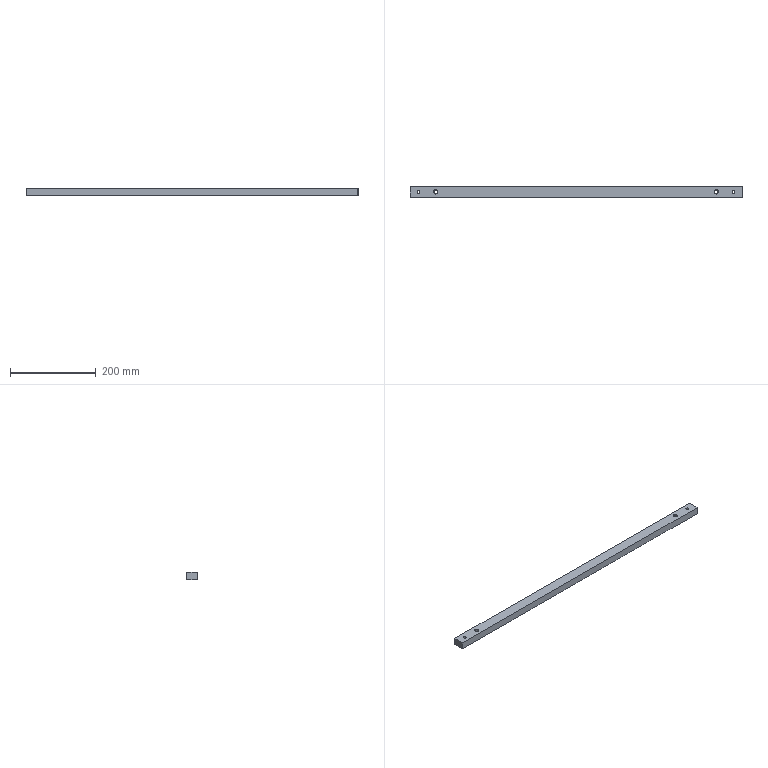Part | NX | features BREP 1 | 1 solid | 48 faces | box 774.5 x 26 x 17 mm | volume 338112 mm3 | cylinder 20 | cone 16 | plane 12 | commonest cylinder face diameters 3.3 x8 6.6 x4 8 x4 11 x4
STEP:
#1=CARTESIAN_POINT('',(372.75,0.,-1.5));
#2=VERTEX_POINT('',#1);
#3=CARTESIAN_POINT('',(361.75,0.,-1.5));
#4=VERTEX_POINT('',#3);
#5=CARTESIAN_POINT('',(367.25,0.,-1.5));
#6=DIRECTION('',(0.,0.,-1.));
#7=DIRECTION('',(-1.,0.,0.));
#8=AXIS2_PLACEMENT_3D('',#5,#6,#7);
#9=CIRCLE('',#8,5.5);
#10=EDGE_CURVE('',#2,#4,#9,.T.);
#11=ORIENTED_EDGE('',*,*,#10,.F.);
#12=CARTESIAN_POINT('',(372.75,0.,-8.5));
#13=VERTEX_POINT('',#12);
#14=CARTESIAN_POINT('',(372.75,0.,-8.5));
#15=DIRECTION('',(0.,0.,-1.));
#16=VECTOR('',#15,1000.);
#17=LINE('',#14,#16);
#18=EDGE_CURVE('',#2,#13,#17,.T.);
#19=ORIENTED_EDGE('',*,*,#18,.T.);
#20=CARTESIAN_POINT('',(361.75,0.,-8.5));
#21=VERTEX_POINT('',#20);
#22=CARTESIAN_POINT('',(367.25,0.,-8.5));
#23=DIRECTION('',(0.,0.,-1.));
#24=DIRECTION('',(-1.,0.,0.));
#25=AXIS2_PLACEMENT_3D('',#22,#23,#24);
#26=CIRCLE('',#25,5.5);
#27=EDGE_CURVE('',#13,#21,#26,.T.);
#28=ORIENTED_EDGE('',*,*,#27,.T.);
#29=CARTESIAN_POINT('',(361.75,0.,-8.5));
#30=DIRECTION('',(0.,0.,-1.));
#31=VECTOR('',#30,1000.);
#32=LINE('',#29,#31);
#33=EDGE_CURVE('',#4,#21,#32,.T.);
#34=ORIENTED_EDGE('',*,*,#33,.F.);
#35=EDGE_LOOP('',(#11,#19,#28,#34));
#36=FACE_BOUND('',#35,.T.);
#37=CARTESIAN_POINT('',(367.25,0.,-8.5));
#38=DIRECTION('',(0.,0.,-1.));
#39=DIRECTION('',(-1.,0.,0.));
#40=AXIS2_PLACEMENT_3D('',#37,#38,#39);
#41=CYLINDRICAL_SURFACE('',#40,5.5);
#42=ADVANCED_FACE('',(#36),#41,.F.);
#43=CARTESIAN_POINT('',(370.55,0.,8.5));
#44=VERTEX_POINT('',#43);
#45=CARTESIAN_POINT('',(363.95,0.,8.5));
#46=VERTEX_POINT('',#45);
#47=CARTESIAN_POINT('',(367.25,0.,8.5));
#48=DIRECTION('',(0.,0.,-1.));
#49=DIRECTION('',(-1.,0.,0.));
#50=AXIS2_PLACEMENT_3D('',#47,#48,#49);
#51=CIRCLE('',#50,3.3);
#52=EDGE_CURVE('',#44,#46,#51,.T.);
#53=ORIENTED_EDGE('',*,*,#52,.F.);
#54=CARTESIAN_POINT('',(370.55,0.,-1.5));
#55=VERTEX_POINT('',#54);
#56=CARTESIAN_POINT('',(370.55,0.,-8.5));
#57=DIRECTION('',(0.,0.,-1.));
#58=VECTOR('',#57,1000.);
#59=LINE('',#56,#58);
#60=EDGE_CURVE('',#44,#55,#59,.T.);
#61=ORIENTED_EDGE('',*,*,#60,.T.);
#62=CARTESIAN_POINT('',(363.95,0.,-1.5));
#63=VERTEX_POINT('',#62);
#64=CARTESIAN_POINT('',(367.25,0.,-1.5));
#65=DIRECTION('',(0.,0.,-1.));
#66=DIRECTION('',(-1.,0.,0.));
#67=AXIS2_PLACEMENT_3D('',#64,#65,#66);
#68=CIRCLE('',#67,3.3);
#69=EDGE_CURVE('',#55,#63,#68,.T.);
#70=ORIENTED_EDGE('',*,*,#69,.T.);
#71=CARTESIAN_POINT('',(363.95,0.,-8.5));
#72=DIRECTION('',(0.,0.,-1.));
#73=VECTOR('',#72,1000.);
#74=LINE('',#71,#73);
#75=EDGE_CURVE('',#46,#63,#74,.T.);
#76=ORIENTED_EDGE('',*,*,#75,.F.);
#77=EDGE_LOOP('',(#53,#61,#70,#76));
#78=FACE_BOUND('',#77,.T.);
#79=CARTESIAN_POINT('',(367.25,0.,-8.5));
#80=DIRECTION('',(0.,0.,-1.));
#81=DIRECTION('',(-1.,0.,0.));
#82=AXIS2_PLACEMENT_3D('',#79,#80,#81);
#83=CYLINDRICAL_SURFACE('',#82,3.3);
#84=ADVANCED_FACE('',(#78),#83,.F.);
#85=CARTESIAN_POINT('',(-361.75,0.,-1.5));
#86=VERTEX_POINT('',#85);
#87=CARTESIAN_POINT('',(-372.75,0.,-1.5));
#88=VERTEX_POINT('',#87);
#89=CARTESIAN_POINT('',(-367.25,0.,-1.5));
#90=DIRECTION('',(0.,0.,-1.));
#91=DIRECTION('',(-1.,0.,0.));
#92=AXIS2_PLACEMENT_3D('',#89,#90,#91);
#93=CIRCLE('',#92,5.5);
#94=EDGE_CURVE('',#86,#88,#93,.T.);
#95=ORIENTED_EDGE('',*,*,#94,.F.);
#96=CARTESIAN_POINT('',(-361.75,0.,-8.5));
#97=VERTEX_POINT('',#96);
#98=CARTESIAN_POINT('',(-361.75,0.,-8.5));
#99=DIRECTION('',(0.,0.,-1.));
#100=VECTOR('',#99,1000.);
#101=LINE('',#98,#100);
#102=EDGE_CURVE('',#86,#97,#101,.T.);
#103=ORIENTED_EDGE('',*,*,#102,.T.);
#104=CARTESIAN_POINT('',(-372.75,0.,-8.5));
#105=VERTEX_POINT('',#104);
#106=CARTESIAN_POINT('',(-367.25,0.,-8.5));
#107=DIRECTION('',(0.,0.,-1.));
#108=DIRECTION('',(-1.,0.,0.));
#109=AXIS2_PLACEMENT_3D('',#106,#107,#108);
#110=CIRCLE('',#109,5.5);
#111=EDGE_CURVE('',#97,#105,#110,.T.);
#112=ORIENTED_EDGE('',*,*,#111,.T.);
#113=CARTESIAN_POINT('',(-372.75,0.,-8.5));
#114=DIRECTION('',(0.,0.,-1.));
#115=VECTOR('',#114,1000.);
#116=LINE('',#113,#115);
#117=EDGE_CURVE('',#88,#105,#116,.T.);
#118=ORIENTED_EDGE('',*,*,#117,.F.);
#119=EDGE_LOOP('',(#95,#103,#112,#118));
#120=FACE_BOUND('',#119,.T.);
#121=CARTESIAN_POINT('',(-367.25,0.,-8.5));
#122=DIRECTION('',(0.,0.,-1.));
#123=DIRECTION('',(-1.,0.,0.));
#124=AXIS2_PLACEMENT_3D('',#121,#122,#123);
#125=CYLINDRICAL_SURFACE('',#124,5.5);
#126=ADVANCED_FACE('',(#120),#125,.F.);
#127=CARTESIAN_POINT('',(-363.95,0.,8.5));
#128=VERTEX_POINT('',#127);
#129=CARTESIAN_POINT('',(-370.55,0.,8.5));
#130=VERTEX_POINT('',#129);
#131=CARTESIAN_POINT('',(-367.25,0.,8.5));
#132=DIRECTION('',(0.,0.,-1.));
#133=DIRECTION('',(-1.,0.,0.));
#134=AXIS2_PLACEMENT_3D('',#131,#132,#133);
#135=CIRCLE('',#134,3.3);
#136=EDGE_CURVE('',#128,#130,#135,.T.);
#137=ORIENTED_EDGE('',*,*,#136,.F.);
#138=CARTESIAN_POINT('',(-363.95,0.,-1.5));
#139=VERTEX_POINT('',#138);
#140=CARTESIAN_POINT('',(-363.95,0.,-8.5));
#141=DIRECTION('',(0.,0.,-1.));
#142=VECTOR('',#141,1000.);
#143=LINE('',#140,#142);
#144=EDGE_CURVE('',#128,#139,#143,.T.);
#145=ORIENTED_EDGE('',*,*,#144,.T.);
#146=CARTESIAN_POINT('',(-370.55,0.,-1.5));
#147=VERTEX_POINT('',#146);
#148=CARTESIAN_POINT('',(-367.25,0.,-1.5));
#149=DIRECTION('',(0.,0.,-1.));
#150=DIRECTION('',(-1.,0.,0.));
#151=AXIS2_PLACEMENT_3D('',#148,#149,#150);
#152=CIRCLE('',#151,3.3);
#153=EDGE_CURVE('',#139,#147,#152,.T.);
#154=ORIENTED_EDGE('',*,*,#153,.T.);
#155=CARTESIAN_POINT('',(-370.55,0.,-8.5));
#156=DIRECTION('',(0.,0.,-1.));
#157=VECTOR('',#156,1000.);
#158=LINE('',#155,#157);
#159=EDGE_CURVE('',#130,#147,#158,.T.);
#160=ORIENTED_EDGE('',*,*,#159,.F.);
#161=EDGE_LOOP('',(#137,#145,#154,#160));
#162=FACE_BOUND('',#161,.T.);
#163=CARTESIAN_POINT('',(-367.25,0.,-8.5));
#164=DIRECTION('',(0.,0.,-1.));
#165=DIRECTION('',(-1.,0.,0.));
#166=AXIS2_PLACEMENT_3D('',#163,#164,#165);
#167=CYLINDRICAL_SURFACE('',#166,3.3);
#168=ADVANCED_FACE('',(#162),#167,.F.);
#169=CARTESIAN_POINT('',(-331.25,0.,7.5));
#170=VERTEX_POINT('',#169);
#171=CARTESIAN_POINT('',(-323.25,0.,7.5));
#172=VERTEX_POINT('',#171);
#173=CARTESIAN_POINT('',(-327.25,0.,7.5));
#174=DIRECTION('',(0.,0.,1.));
#175=DIRECTION('',(-1.,0.,0.));
#176=AXIS2_PLACEMENT_3D('',#173,#174,#175);
#177=CIRCLE('',#176,4.);
#178=EDGE_CURVE('',#170,#172,#177,.T.);
#179=ORIENTED_EDGE('',*,*,#178,.F.);
#180=CARTESIAN_POINT('',(-332.25,0.,8.5));
#181=VERTEX_POINT('',#180);
#182=CARTESIAN_POINT('',(-331.25,0.,7.5));
#183=DIRECTION('',(-0.7071,0.,0.7071));
#184=VECTOR('',#183,1000.);
#185=LINE('',#182,#184);
#186=EDGE_CURVE('',#181,#170,#185,.F.);
#187=ORIENTED_EDGE('',*,*,#186,.F.);
#188=CARTESIAN_POINT('',(-322.25,0.,8.5));
#189=VERTEX_POINT('',#188);
#190=CARTESIAN_POINT('',(-327.25,0.,8.5));
#191=DIRECTION('',(0.,0.,-1.));
#192=DIRECTION('',(-1.,0.,0.));
#193=AXIS2_PLACEMENT_3D('',#190,#191,#192);
#194=CIRCLE('',#193,5.);
#195=EDGE_CURVE('',#189,#181,#194,.T.);
#196=ORIENTED_EDGE('',*,*,#195,.F.);
#197=CARTESIAN_POINT('',(-323.25,0.,7.5));
#198=DIRECTION('',(0.7071,0.,0.7071));
#199=VECTOR('',#198,1000.);
#200=LINE('',#197,#199);
#201=EDGE_CURVE('',#189,#172,#200,.F.);
#202=ORIENTED_EDGE('',*,*,#201,.T.);
#203=EDGE_LOOP('',(#179,#187,#196,#202));
#204=FACE_BOUND('',#203,.T.);
#205=CARTESIAN_POINT('',(-327.25,0.,7.5));
#206=DIRECTION('',(0.,0.,1.));
#207=DIRECTION('',(1.,0.,0.));
#208=AXIS2_PLACEMENT_3D('',#205,#206,#207);
#209=CONICAL_SURFACE('',#208,4.,0.7854);
#210=ADVANCED_FACE('',(#204),#209,.F.);
#211=CARTESIAN_POINT('',(-323.25,0.,-7.5));
#212=VERTEX_POINT('',#211);
#213=CARTESIAN_POINT('',(-331.25,0.,-7.5));
#214=VERTEX_POINT('',#213);
#215=CARTESIAN_POINT('',(-327.25,0.,-7.5));
#216=DIRECTION('',(0.,0.,-1.));
#217=DIRECTION('',(-1.,0.,0.));
#218=AXIS2_PLACEMENT_3D('',#215,#216,#217);
#219=CIRCLE('',#218,4.);
#220=EDGE_CURVE('',#212,#214,#219,.T.);
#221=ORIENTED_EDGE('',*,*,#220,.F.);
#222=CARTESIAN_POINT('',(-322.25,0.,-8.5));
#223=VERTEX_POINT('',#222);
#224=CARTESIAN_POINT('',(-323.25,0.,-7.5));
#225=DIRECTION('',(0.7071,0.,-0.7071));
#226=VECTOR('',#225,1000.);
#227=LINE('',#224,#226);
#228=EDGE_CURVE('',#212,#223,#227,.T.);
#229=ORIENTED_EDGE('',*,*,#228,.T.);
#230=CARTESIAN_POINT('',(-332.25,0.,-8.5));
#231=VERTEX_POINT('',#230);
#232=CARTESIAN_POINT('',(-327.25,0.,-8.5));
#233=DIRECTION('',(0.,0.,1.));
#234=DIRECTION('',(-1.,0.,0.));
#235=AXIS2_PLACEMENT_3D('',#232,#233,#234);
#236=CIRCLE('',#235,5.);
#237=EDGE_CURVE('',#231,#223,#236,.T.);
#238=ORIENTED_EDGE('',*,*,#237,.F.);
#239=CARTESIAN_POINT('',(-331.25,0.,-7.5));
#240=DIRECTION('',(-0.7071,0.,-0.7071));
#241=VECTOR('',#240,1000.);
#242=LINE('',#239,#241);
#243=EDGE_CURVE('',#214,#231,#242,.T.);
#244=ORIENTED_EDGE('',*,*,#243,.F.);
#245=EDGE_LOOP('',(#221,#229,#238,#244));
#246=FACE_BOUND('',#245,.T.);
#247=CARTESIAN_POINT('',(-327.25,0.,-7.5));
#248=DIRECTION('',(0.,0.,-1.));
#249=DIRECTION('',(-1.,0.,0.));
#250=AXIS2_PLACEMENT_3D('',#247,#248,#249);
#251=CONICAL_SURFACE('',#250,4.,0.7854);
#252=ADVANCED_FACE('',(#246),#251,.F.);
#253=CARTESIAN_POINT('',(323.25,0.,7.5));
#254=VERTEX_POINT('',#253);
#255=CARTESIAN_POINT('',(331.25,0.,7.5));
#256=VERTEX_POINT('',#255);
#257=CARTESIAN_POINT('',(327.25,0.,7.5));
#258=DIRECTION('',(0.,0.,1.));
#259=DIRECTION('',(-1.,0.,0.));
#260=AXIS2_PLACEMENT_3D('',#257,#258,#259);
#261=CIRCLE('',#260,4.);
#262=EDGE_CURVE('',#254,#256,#261,.T.);
#263=ORIENTED_EDGE('',*,*,#262,.F.);
#264=CARTESIAN_POINT('',(322.25,0.,8.5));
#265=VERTEX_POINT('',#264);
#266=CARTESIAN_POINT('',(323.25,0.,7.5));
#267=DIRECTION('',(-0.7071,0.,0.7071));
#268=VECTOR('',#267,1000.);
#269=LINE('',#266,#268);
#270=EDGE_CURVE('',#265,#254,#269,.F.);
#271=ORIENTED_EDGE('',*,*,#270,.F.);
#272=CARTESIAN_POINT('',(332.25,0.,8.5));
#273=VERTEX_POINT('',#272);
#274=CARTESIAN_POINT('',(327.25,0.,8.5));
#275=DIRECTION('',(0.,0.,-1.));
#276=DIRECTION('',(-1.,0.,0.));
#277=AXIS2_PLACEMENT_3D('',#274,#275,#276);
#278=CIRCLE('',#277,5.);
#279=EDGE_CURVE('',#273,#265,#278,.T.);
#280=ORIENTED_EDGE('',*,*,#279,.F.);
#281=CARTESIAN_POINT('',(331.25,0.,7.5));
#282=DIRECTION('',(0.7071,0.,0.7071));
#283=VECTOR('',#282,1000.);
#284=LINE('',#281,#283);
#285=EDGE_CURVE('',#273,#256,#284,.F.);
#286=ORIENTED_EDGE('',*,*,#285,.T.);
#287=EDGE_LOOP('',(#263,#271,#280,#286));
#288=FACE_BOUND('',#287,.T.);
#289=CARTESIAN_POINT('',(327.25,0.,7.5));
#290=DIRECTION('',(0.,0.,1.));
#291=DIRECTION('',(1.,0.,0.));
#292=AXIS2_PLACEMENT_3D('',#289,#290,#291);
#293=CONICAL_SURFACE('',#292,4.,0.7854);
#294=ADVANCED_FACE('',(#288),#293,.F.);
#295=CARTESIAN_POINT('',(331.25,0.,-7.5));
#296=VERTEX_POINT('',#295);
#297=CARTESIAN_POINT('',(323.25,0.,-7.5));
#298=VERTEX_POINT('',#297);
#299=CARTESIAN_POINT('',(327.25,0.,-7.5));
#300=DIRECTION('',(0.,0.,-1.));
#301=DIRECTION('',(-1.,0.,0.));
#302=AXIS2_PLACEMENT_3D('',#299,#300,#301);
#303=CIRCLE('',#302,4.);
#304=EDGE_CURVE('',#296,#298,#303,.T.);
#305=ORIENTED_EDGE('',*,*,#304,.F.);
#306=CARTESIAN_POINT('',(332.25,0.,-8.5));
#307=VERTEX_POINT('',#306);
#308=CARTESIAN_POINT('',(331.25,0.,-7.5));
#309=DIRECTION('',(0.7071,0.,-0.7071));
#310=VECTOR('',#309,1000.);
#311=LINE('',#308,#310);
#312=EDGE_CURVE('',#296,#307,#311,.T.);
#313=ORIENTED_EDGE('',*,*,#312,.T.);
#314=CARTESIAN_POINT('',(322.25,0.,-8.5));
#315=VERTEX_POINT('',#314);
#316=CARTESIAN_POINT('',(327.25,0.,-8.5));
#317=DIRECTION('',(0.,0.,1.));
#318=DIRECTION('',(-1.,0.,0.));
#319=AXIS2_PLACEMENT_3D('',#316,#317,#318);
#320=CIRCLE('',#319,5.);
#321=EDGE_CURVE('',#315,#307,#320,.T.);
#322=ORIENTED_EDGE('',*,*,#321,.F.);
#323=CARTESIAN_POINT('',(323.25,0.,-7.5));
#324=DIRECTION('',(-0.7071,0.,-0.7071));
#325=VECTOR('',#324,1000.);
#326=LINE('',#323,#325);
#327=EDGE_CURVE('',#298,#315,#326,.T.);
#328=ORIENTED_EDGE('',*,*,#327,.F.);
#329=EDGE_LOOP('',(#305,#313,#322,#328));
#330=FACE_BOUND('',#329,.T.);
#331=CARTESIAN_POINT('',(327.25,0.,-7.5));
#332=DIRECTION('',(0.,0.,-1.));
#333=DIRECTION('',(-1.,0.,0.));
#334=AXIS2_PLACEMENT_3D('',#331,#332,#333);
#335=CONICAL_SURFACE('',#334,4.,0.7854);
#336=ADVANCED_FACE('',(#330),#335,.F.);
#337=ORIENTED_EDGE('',*,*,#304,.T.);
#338=CARTESIAN_POINT('',(323.25,0.,-174.5));
#339=DIRECTION('',(0.,0.,1.));
#340=VECTOR('',#339,1000.);
#341=LINE('',#338,#340);
#342=EDGE_CURVE('',#254,#298,#341,.F.);
#343=ORIENTED_EDGE('',*,*,#342,.F.);
#344=ORIENTED_EDGE('',*,*,#262,.T.);
#345=CARTESIAN_POINT('',(331.25,0.,-174.5));
#346=DIRECTION('',(0.,0.,1.));
#347=VECTOR('',#346,1000.);
#348=LINE('',#345,#347);
#349=EDGE_CURVE('',#256,#296,#348,.F.);
#350=ORIENTED_EDGE('',*,*,#349,.T.);
#351=EDGE_LOOP('',(#337,#343,#344,#350));
#352=FACE_BOUND('',#351,.T.);
#353=CARTESIAN_POINT('',(327.25,0.,-174.5));
#354=DIRECTION('',(0.,0.,1.));
#355=DIRECTION('',(1.,0.,0.));
#356=AXIS2_PLACEMENT_3D('',#353,#354,#355);
#357=CYLINDRICAL_SURFACE('',#356,4.);
#358=ADVANCED_FACE('',(#352),#357,.F.);
#359=ORIENTED_EDGE('',*,*,#220,.T.);
#360=CARTESIAN_POINT('',(-331.25,0.,-174.5));
#361=DIRECTION('',(0.,0.,1.));
#362=VECTOR('',#361,1000.);
#363=LINE('',#360,#362);
#364=EDGE_CURVE('',#170,#214,#363,.F.);
#365=ORIENTED_EDGE('',*,*,#364,.F.);
#366=ORIENTED_EDGE('',*,*,#178,.T.);
#367=CARTESIAN_POINT('',(-323.25,0.,-174.5));
#368=DIRECTION('',(0.,0.,1.));
#369=VECTOR('',#368,1000.);
#370=LINE('',#367,#369);
#371=EDGE_CURVE('',#172,#212,#370,.F.);
#372=ORIENTED_EDGE('',*,*,#371,.T.);
#373=EDGE_LOOP('',(#359,#365,#366,#372));
#374=FACE_BOUND('',#373,.T.);
#375=CARTESIAN_POINT('',(-327.25,0.,-174.5));
#376=DIRECTION('',(0.,0.,1.));
#377=DIRECTION('',(1.,0.,0.));
#378=AXIS2_PLACEMENT_3D('',#375,#376,#377);
#379=CYLINDRICAL_SURFACE('',#378,4.);
#380=ADVANCED_FACE('',(#374),#379,.F.);
#381=CARTESIAN_POINT('',(-374.25,1.5,-1.65));
#382=VERTEX_POINT('',#381);
#383=CARTESIAN_POINT('',(-374.25,1.5,1.65));
#384=VERTEX_POINT('',#383);
#385=CARTESIAN_POINT('',(-374.25,1.5,0.));
#386=DIRECTION('',(0.,1.,0.));
#387=DIRECTION('',(0.,0.,1.));
#388=AXIS2_PLACEMENT_3D('',#385,#386,#387);
#389=CIRCLE('',#388,1.65);
#390=EDGE_CURVE('',#382,#384,#389,.T.);
#391=ORIENTED_EDGE('',*,*,#390,.F.);
#392=CARTESIAN_POINT('',(-374.25,13.,-1.65));
#393=VERTEX_POINT('',#392);
#394=CARTESIAN_POINT('',(-374.25,13.,-1.65));
#395=DIRECTION('',(0.,1.,0.));
#396=VECTOR('',#395,1000.);
#397=LINE('',#394,#396);
#398=EDGE_CURVE('',#393,#382,#397,.F.);
#399=ORIENTED_EDGE('',*,*,#398,.F.);
#400=CARTESIAN_POINT('',(-374.25,13.,1.65));
#401=VERTEX_POINT('',#400);
#402=CARTESIAN_POINT('',(-374.25,13.,0.));
#403=DIRECTION('',(0.,1.,0.));
#404=DIRECTION('',(0.,0.,1.));
#405=AXIS2_PLACEMENT_3D('',#402,#403,#404);
#406=CIRCLE('',#405,1.65);
#407=EDGE_CURVE('',#393,#401,#406,.T.);
#408=ORIENTED_EDGE('',*,*,#407,.T.);
#409=CARTESIAN_POINT('',(-374.25,13.,1.65));
#410=DIRECTION('',(0.,1.,0.));
#411=VECTOR('',#410,1000.);
#412=LINE('',#409,#411);
#413=EDGE_CURVE('',#401,#384,#412,.F.);
#414=ORIENTED_EDGE('',*,*,#413,.T.);
#415=EDGE_LOOP('',(#391,#399,#408,#414));
#416=FACE_BOUND('',#415,.T.);
#417=CARTESIAN_POINT('',(-374.25,13.,0.));
#418=DIRECTION('',(0.,1.,0.));
#419=DIRECTION('',(0.,0.,1.));
#420=AXIS2_PLACEMENT_3D('',#417,#418,#419);
#421=CYLINDRICAL_SURFACE('',#420,1.65);
#422=ADVANCED_FACE('',(#416),#421,.F.);
#423=CARTESIAN_POINT('',(-374.25,0.5086,0.));
#424=VERTEX_POINT('',#423);
#425=CARTESIAN_POINT('',(-374.25,1.5,1.65));
#426=DIRECTION('',(0.,0.515,0.8572));
#427=VECTOR('',#426,1000.);
#428=LINE('',#425,#427);
#429=EDGE_CURVE('',#384,#424,#428,.F.);
#430=ORIENTED_EDGE('',*,*,#429,.T.);
#431=CARTESIAN_POINT('',(-374.25,1.5,-1.65));
#432=DIRECTION('',(0.,0.515,-0.8572));
#433=VECTOR('',#432,1000.);
#434=LINE('',#431,#433);
#435=EDGE_CURVE('',#382,#424,#434,.F.);
#436=ORIENTED_EDGE('',*,*,#435,.F.);
#437=ORIENTED_EDGE('',*,*,#390,.T.);
#438=EDGE_LOOP('',(#430,#436,#437));
#439=FACE_BOUND('',#438,.T.);
#440=CARTESIAN_POINT('',(-374.25,1.5,0.));
#441=DIRECTION('',(0.,1.,0.));
#442=DIRECTION('',(0.,0.,1.));
#443=AXIS2_PLACEMENT_3D('',#440,#441,#442);
#444=CONICAL_SURFACE('',#443,1.65,1.03);
#445=ADVANCED_FACE('',(#439),#444,.F.);
#446=CARTESIAN_POINT('',(-137.25,1.5,-1.65));
#447=VERTEX_POINT('',#446);
#448=CARTESIAN_POINT('',(-137.25,1.5,1.65));
#449=VERTEX_POINT('',#448);
#450=CARTESIAN_POINT('',(-137.25,1.5,0.));
#451=DIRECTION('',(0.,1.,0.));
#452=DIRECTION('',(0.,0.,1.));
#453=AXIS2_PLACEMENT_3D('',#450,#451,#452);
#454=CIRCLE('',#453,1.65);
#455=EDGE_CURVE('',#447,#449,#454,.T.);
#456=ORIENTED_EDGE('',*,*,#455,.F.);
#457=CARTESIAN_POINT('',(-137.25,13.,-1.65));
#458=VERTEX_POINT('',#457);
#459=CARTESIAN_POINT('',(-137.25,13.,-1.65));
#460=DIRECTION('',(0.,1.,0.));
#461=VECTOR('',#460,1000.);
#462=LINE('',#459,#461);
#463=EDGE_CURVE('',#458,#447,#462,.F.);
#464=ORIENTED_EDGE('',*,*,#463,.F.);
#465=CARTESIAN_POINT('',(-137.25,13.,1.65));
#466=VERTEX_POINT('',#465);
#467=CARTESIAN_POINT('',(-137.25,13.,0.));
#468=DIRECTION('',(0.,1.,0.));
#469=DIRECTION('',(0.,0.,1.));
#470=AXIS2_PLACEMENT_3D('',#467,#468,#469);
#471=CIRCLE('',#470,1.65);
#472=EDGE_CURVE('',#458,#466,#471,.T.);
#473=ORIENTED_EDGE('',*,*,#472,.T.);
#474=CARTESIAN_POINT('',(-137.25,13.,1.65));
#475=DIRECTION('',(0.,1.,0.));
#476=VECTOR('',#475,1000.);
#477=LINE('',#474,#476);
#478=EDGE_CURVE('',#466,#449,#477,.F.);
#479=ORIENTED_EDGE('',*,*,#478,.T.);
#480=EDGE_LOOP('',(#456,#464,#473,#479));
#481=FACE_BOUND('',#480,.T.);
#482=CARTESIAN_POINT('',(-137.25,13.,0.));
#483=DIRECTION('',(0.,1.,0.));
#484=DIRECTION('',(0.,0.,1.));
#485=AXIS2_PLACEMENT_3D('',#482,#483,#484);
#486=CYLINDRICAL_SURFACE('',#485,1.65);
#487=ADVANCED_FACE('',(#481),#486,.F.);
#488=CARTESIAN_POINT('',(-137.25,0.5086,0.));
#489=VERTEX_POINT('',#488);
#490=CARTESIAN_POINT('',(-137.25,1.5,1.65));
#491=DIRECTION('',(0.,0.515,0.8572));
#492=VECTOR('',#491,1000.);
#493=LINE('',#490,#492);
#494=EDGE_CURVE('',#449,#489,#493,.F.);
#495=ORIENTED_EDGE('',*,*,#494,.T.);
#496=CARTESIAN_POINT('',(-137.25,1.5,-1.65));
#497=DIRECTION('',(0.,0.515,-0.8572));
#498=VECTOR('',#497,1000.);
#499=LINE('',#496,#498);
#500=EDGE_CURVE('',#447,#489,#499,.F.);
#501=ORIENTED_EDGE('',*,*,#500,.F.);
#502=ORIENTED_EDGE('',*,*,#455,.T.);
#503=EDGE_LOOP('',(#495,#501,#502));
#504=FACE_BOUND('',#503,.T.);
#505=CARTESIAN_POINT('',(-137.25,1.5,0.));
#506=DIRECTION('',(0.,1.,0.));
#507=DIRECTION('',(0.,0.,1.));
#508=AXIS2_PLACEMENT_3D('',#505,#506,#507);
#509=CONICAL_SURFACE('',#508,1.65,1.03);
#510=ADVANCED_FACE('',(#504),#509,.F.);
#511=CARTESIAN_POINT('',(99.75,1.5,-1.65));
#512=VERTEX_POINT('',#511);
#513=CARTESIAN_POINT('',(99.75,1.5,1.65));
#514=VERTEX_POINT('',#513);
#515=CARTESIAN_POINT('',(99.75,1.5,0.));
#516=DIRECTION('',(0.,1.,0.));
#517=DIRECTION('',(0.,0.,1.));
#518=AXIS2_PLACEMENT_3D('',#515,#516,#517);
#519=CIRCLE('',#518,1.65);
#520=EDGE_CURVE('',#512,#514,#519,.T.);
#521=ORIENTED_EDGE('',*,*,#520,.F.);
#522=CARTESIAN_POINT('',(99.75,13.,-1.65));
#523=VERTEX_POINT('',#522);
#524=CARTESIAN_POINT('',(99.75,13.,-1.65));
#525=DIRECTION('',(0.,1.,0.));
#526=VECTOR('',#525,1000.);
#527=LINE('',#524,#526);
#528=EDGE_CURVE('',#523,#512,#527,.F.);
#529=ORIENTED_EDGE('',*,*,#528,.F.);
#530=CARTESIAN_POINT('',(99.75,13.,1.65));
#531=VERTEX_POINT('',#530);
#532=CARTESIAN_POINT('',(99.75,13.,0.));
#533=DIRECTION('',(0.,1.,0.));
#534=DIRECTION('',(0.,0.,1.));
#535=AXIS2_PLACEMENT_3D('',#532,#533,#534);
#536=CIRCLE('',#535,1.65);
#537=EDGE_CURVE('',#523,#531,#536,.T.);
#538=ORIENTED_EDGE('',*,*,#537,.T.);
#539=CARTESIAN_POINT('',(99.75,13.,1.65));
#540=DIRECTION('',(0.,1.,0.));
#541=VECTOR('',#540,1000.);
#542=LINE('',#539,#541);
#543=EDGE_CURVE('',#531,#514,#542,.F.);
#544=ORIENTED_EDGE('',*,*,#543,.T.);
#545=EDGE_LOOP('',(#521,#529,#538,#544));
#546=FACE_BOUND('',#545,.T.);
#547=CARTESIAN_POINT('',(99.75,13.,0.));
#548=DIRECTION('',(0.,1.,0.));
#549=DIRECTION('',(0.,0.,1.));
#550=AXIS2_PLACEMENT_3D('',#547,#548,#549);
#551=CYLINDRICAL_SURFACE('',#550,1.65);
#552=ADVANCED_FACE('',(#546),#551,.F.);
#553=CARTESIAN_POINT('',(99.75,0.5086,0.));
#554=VERTEX_POINT('',#553);
#555=CARTESIAN_POINT('',(99.75,1.5,1.65));
#556=DIRECTION('',(0.,0.515,0.8572));
#557=VECTOR('',#556,1000.);
#558=LINE('',#555,#557);
#559=EDGE_CURVE('',#514,#554,#558,.F.);
#560=ORIENTED_EDGE('',*,*,#559,.T.);
#561=CARTESIAN_POINT('',(99.75,1.5,-1.65));
#562=DIRECTION('',(0.,0.515,-0.8572));
#563=VECTOR('',#562,1000.);
#564=LINE('',#561,#563);
#565=EDGE_CURVE('',#512,#554,#564,.F.);
#566=ORIENTED_EDGE('',*,*,#565,.F.);
#567=ORIENTED_EDGE('',*,*,#520,.T.);
#568=EDGE_LOOP('',(#560,#566,#567));
#569=FACE_BOUND('',#568,.T.);
#570=CARTESIAN_POINT('',(99.75,1.5,0.));
#571=DIRECTION('',(0.,1.,0.));
#572=DIRECTION('',(0.,0.,1.));
#573=AXIS2_PLACEMENT_3D('',#570,#571,#572);
#574=CONICAL_SURFACE('',#573,1.65,1.03);
#575=ADVANCED_FACE('',(#569),#574,.F.);
#576=CARTESIAN_POINT('',(336.75,1.5,-1.65));
#577=VERTEX_POINT('',#576);
#578=CARTESIAN_POINT('',(336.75,1.5,1.65));
#579=VERTEX_POINT('',#578);
#580=CARTESIAN_POINT('',(336.75,1.5,0.));
#581=DIRECTION('',(0.,1.,0.));
#582=DIRECTION('',(0.,0.,1.));
#583=AXIS2_PLACEMENT_3D('',#580,#581,#582);
#584=CIRCLE('',#583,1.65);
#585=EDGE_CURVE('',#577,#579,#584,.T.);
#586=ORIENTED_EDGE('',*,*,#585,.F.);
#587=CARTESIAN_POINT('',(336.75,13.,-1.65));
#588=VERTEX_POINT('',#587);
#589=CARTESIAN_POINT('',(336.75,13.,-1.65));
#590=DIRECTION('',(0.,1.,0.));
#591=VECTOR('',#590,1000.);
#592=LINE('',#589,#591);
#593=EDGE_CURVE('',#588,#577,#592,.F.);
#594=ORIENTED_EDGE('',*,*,#593,.F.);
#595=CARTESIAN_POINT('',(336.75,13.,1.65));
#596=VERTEX_POINT('',#595);
#597=CARTESIAN_POINT('',(336.75,13.,0.));
#598=DIRECTION('',(0.,1.,0.));
#599=DIRECTION('',(0.,0.,1.));
#600=AXIS2_PLACEMENT_3D('',#597,#598,#599);
#601=CIRCLE('',#600,1.65);
#602=EDGE_CURVE('',#588,#596,#601,.T.);
#603=ORIENTED_EDGE('',*,*,#602,.T.);
#604=CARTESIAN_POINT('',(336.75,13.,1.65));
#605=DIRECTION('',(0.,1.,0.));
#606=VECTOR('',#605,1000.);
#607=LINE('',#604,#606);
#608=EDGE_CURVE('',#596,#579,#607,.F.);
#609=ORIENTED_EDGE('',*,*,#608,.T.);
#610=EDGE_LOOP('',(#586,#594,#603,#609));
#611=FACE_BOUND('',#610,.T.);
#612=CARTESIAN_POINT('',(336.75,13.,0.));
#613=DIRECTION('',(0.,1.,0.));
#614=DIRECTION('',(0.,0.,1.));
#615=AXIS2_PLACEMENT_3D('',#612,#613,#614);
#616=CYLINDRICAL_SURFACE('',#615,1.65);
#617=ADVANCED_FACE('',(#611),#616,.F.);
#618=CARTESIAN_POINT('',(336.75,0.5086,0.));
#619=VERTEX_POINT('',#618);
#620=CARTESIAN_POINT('',(336.75,1.5,1.65));
#621=DIRECTION('',(0.,0.515,0.8572));
#622=VECTOR('',#621,1000.);
#623=LINE('',#620,#622);
#624=EDGE_CURVE('',#579,#619,#623,.F.);
#625=ORIENTED_EDGE('',*,*,#624,.T.);
#626=CARTESIAN_POINT('',(336.75,1.5,-1.65));
#627=DIRECTION('',(0.,0.515,-0.8572));
#628=VECTOR('',#627,1000.);
#629=LINE('',#626,#628);
#630=EDGE_CURVE('',#577,#619,#629,.F.);
#631=ORIENTED_EDGE('',*,*,#630,.F.);
#632=ORIENTED_EDGE('',*,*,#585,.T.);
#633=EDGE_LOOP('',(#625,#631,#632));
#634=FACE_BOUND('',#633,.T.);
#635=CARTESIAN_POINT('',(336.75,1.5,0.));
#636=DIRECTION('',(0.,1.,0.));
#637=DIRECTION('',(0.,0.,1.));
#638=AXIS2_PLACEMENT_3D('',#635,#636,#637);
#639=CONICAL_SURFACE('',#638,1.65,1.03);
#640=ADVANCED_FACE('',(#634),#639,.F.);
#641=CARTESIAN_POINT('',(387.25,-12.,8.5));
#642=VERTEX_POINT('',#641);
#643=CARTESIAN_POINT('',(387.25,12.,8.5));
#644=VERTEX_POINT('',#643);
#645=CARTESIAN_POINT('',(387.25,-13.,8.5));
#646=DIRECTION('',(0.,1.,0.));
#647=VECTOR('',#646,1000.);
#648=LINE('',#645,#647);
#649=EDGE_CURVE('',#642,#644,#648,.T.);
#650=ORIENTED_EDGE('',*,*,#649,.F.);
#651=CARTESIAN_POINT('',(387.25,-12.,-8.5));
#652=VERTEX_POINT('',#651);
#653=CARTESIAN_POINT('',(387.25,-12.,8.5));
#654=DIRECTION('',(0.,0.,-1.));
#655=VECTOR('',#654,1000.);
#656=LINE('',#653,#655);
#657=EDGE_CURVE('',#642,#652,#656,.T.);
#658=ORIENTED_EDGE('',*,*,#657,.T.);
#659=CARTESIAN_POINT('',(387.25,12.,-8.5));
#660=VERTEX_POINT('',#659);
#661=CARTESIAN_POINT('',(387.25,-13.,-8.5));
#662=DIRECTION('',(0.,1.,0.));
#663=VECTOR('',#662,1000.);
#664=LINE('',#661,#663);
#665=EDGE_CURVE('',#652,#660,#664,.T.);
#666=ORIENTED_EDGE('',*,*,#665,.T.);
#667=CARTESIAN_POINT('',(387.25,12.,8.5));
#668=DIRECTION('',(0.,0.,1.));
#669=VECTOR('',#668,1000.);
#670=LINE('',#667,#669);
#671=EDGE_CURVE('',#660,#644,#670,.T.);
#672=ORIENTED_EDGE('',*,*,#671,.T.);
#673=EDGE_LOOP('',(#650,#658,#666,#672));
#674=FACE_BOUND('',#673,.T.);
#675=CARTESIAN_POINT('',(387.25,-13.,8.5));
#676=DIRECTION('',(-1.,0.,0.));
#677=DIRECTION('',(0.,0.,1.));
#678=AXIS2_PLACEMENT_3D('',#675,#676,#677);
#679=PLANE('',#678);
#680=ADVANCED_FACE('',(#674),#679,.F.);
#681=CARTESIAN_POINT('',(386.25,13.,8.5));
#682=VERTEX_POINT('',#681);
#683=CARTESIAN_POINT('',(-386.25,13.,8.5));
#684=VERTEX_POINT('',#683);
#685=CARTESIAN_POINT('',(-387.25,13.,8.5));
#686=DIRECTION('',(-1.,0.,0.));
#687=VECTOR('',#686,1000.);
#688=LINE('',#685,#687);
#689=EDGE_CURVE('',#682,#684,#688,.T.);
#690=ORIENTED_EDGE('',*,*,#689,.F.);
#691=CARTESIAN_POINT('',(386.25,13.,-8.5));
#692=VERTEX_POINT('',#691);
#693=CARTESIAN_POINT('',(386.25,13.,8.5));
#694=DIRECTION('',(0.,0.,-1.));
#695=VECTOR('',#694,1000.);
#696=LINE('',#693,#695);
#697=EDGE_CURVE('',#682,#692,#696,.T.);
#698=ORIENTED_EDGE('',*,*,#697,.T.);
#699=CARTESIAN_POINT('',(-386.25,13.,-8.5));
#700=VERTEX_POINT('',#699);
#701=CARTESIAN_POINT('',(-387.25,13.,-8.5));
#702=DIRECTION('',(-1.,0.,0.));
#703=VECTOR('',#702,1000.);
#704=LINE('',#701,#703);
#705=EDGE_CURVE('',#692,#700,#704,.T.);
#706=ORIENTED_EDGE('',*,*,#705,.T.);
#707=CARTESIAN_POINT('',(-386.25,13.,8.5));
#708=DIRECTION('',(0.,0.,1.));
#709=VECTOR('',#708,1000.);
#710=LINE('',#707,#709);
#711=EDGE_CURVE('',#700,#684,#710,.T.);
#712=ORIENTED_EDGE('',*,*,#711,.T.);
#713=EDGE_LOOP('',(#690,#698,#706,#712));
#714=FACE_BOUND('',#713,.T.);
#715=CARTESIAN_POINT('',(-374.25,13.,0.));
#716=DIRECTION('',(0.,1.,0.));
#717=DIRECTION('',(0.,0.,1.));
#718=AXIS2_PLACEMENT_3D('',#715,#716,#717);
#719=CIRCLE('',#718,1.65);
#720=EDGE_CURVE('',#401,#393,#719,.T.);
#721=ORIENTED_EDGE('',*,*,#720,.F.);
#722=ORIENTED_EDGE('',*,*,#407,.F.);
#723=EDGE_LOOP('',(#721,#722));
#724=FACE_BOUND('',#723,.T.);
#725=CARTESIAN_POINT('',(-137.25,13.,0.));
#726=DIRECTION('',(0.,1.,0.));
#727=DIRECTION('',(0.,0.,1.));
#728=AXIS2_PLACEMENT_3D('',#725,#726,#727);
#729=CIRCLE('',#728,1.65);
#730=EDGE_CURVE('',#466,#458,#729,.T.);
#731=ORIENTED_EDGE('',*,*,#730,.F.);
#732=ORIENTED_EDGE('',*,*,#472,.F.);
#733=EDGE_LOOP('',(#731,#732));
#734=FACE_BOUND('',#733,.T.);
#735=CARTESIAN_POINT('',(99.75,13.,0.));
#736=DIRECTION('',(0.,1.,0.));
#737=DIRECTION('',(0.,0.,1.));
#738=AXIS2_PLACEMENT_3D('',#735,#736,#737);
#739=CIRCLE('',#738,1.65);
#740=EDGE_CURVE('',#531,#523,#739,.T.);
#741=ORIENTED_EDGE('',*,*,#740,.F.);
#742=ORIENTED_EDGE('',*,*,#537,.F.);
#743=EDGE_LOOP('',(#741,#742));
#744=FACE_BOUND('',#743,.T.);
#745=CARTESIAN_POINT('',(336.75,13.,0.));
#746=DIRECTION('',(0.,1.,0.));
#747=DIRECTION('',(0.,0.,1.));
#748=AXIS2_PLACEMENT_3D('',#745,#746,#747);
#749=CIRCLE('',#748,1.65);
#750=EDGE_CURVE('',#596,#588,#749,.T.);
#751=ORIENTED_EDGE('',*,*,#750,.F.);
#752=ORIENTED_EDGE('',*,*,#602,.F.);
#753=EDGE_LOOP('',(#751,#752));
#754=FACE_BOUND('',#753,.T.);
#755=CARTESIAN_POINT('',(-387.25,13.,8.5));
#756=DIRECTION('',(0.,-1.,0.));
#757=DIRECTION('',(0.,0.,-1.));
#758=AXIS2_PLACEMENT_3D('',#755,#756,#757);
#759=PLANE('',#758);
#760=ADVANCED_FACE('',(#714,#724,#734,#744,#754),#759,.F.);
#761=CARTESIAN_POINT('',(-387.25,12.,-8.5));
#762=VERTEX_POINT('',#761);
#763=CARTESIAN_POINT('',(-387.25,-12.,-8.5));
#764=VERTEX_POINT('',#763);
#765=CARTESIAN_POINT('',(-387.25,-13.,-8.5));
#766=DIRECTION('',(0.,-1.,0.));
#767=VECTOR('',#766,1000.);
#768=LINE('',#765,#767);
#769=EDGE_CURVE('',#762,#764,#768,.T.);
#770=ORIENTED_EDGE('',*,*,#769,.T.);
#771=CARTESIAN_POINT('',(-387.25,-12.,8.5));
#772=VERTEX_POINT('',#771);
#773=CARTESIAN_POINT('',(-387.25,-12.,8.5));
#774=DIRECTION('',(0.,0.,1.));
#775=VECTOR('',#774,1000.);
#776=LINE('',#773,#775);
#777=EDGE_CURVE('',#764,#772,#776,.T.);
#778=ORIENTED_EDGE('',*,*,#777,.T.);
#779=CARTESIAN_POINT('',(-387.25,12.,8.5));
#780=VERTEX_POINT('',#779);
#781=CARTESIAN_POINT('',(-387.25,-13.,8.5));
#782=DIRECTION('',(0.,-1.,0.));
#783=VECTOR('',#782,1000.);
#784=LINE('',#781,#783);
#785=EDGE_CURVE('',#780,#772,#784,.T.);
#786=ORIENTED_EDGE('',*,*,#785,.F.);
#787=CARTESIAN_POINT('',(-387.25,12.,8.5));
#788=DIRECTION('',(0.,0.,-1.));
#789=VECTOR('',#788,1000.);
#790=LINE('',#787,#789);
#791=EDGE_CURVE('',#780,#762,#790,.T.);
#792=ORIENTED_EDGE('',*,*,#791,.T.);
#793=EDGE_LOOP('',(#770,#778,#786,#792));
#794=FACE_BOUND('',#793,.T.);
#795=CARTESIAN_POINT('',(-387.25,-13.,8.5));
#796=DIRECTION('',(1.,0.,0.));
#797=DIRECTION('',(0.,1.,0.));
#798=AXIS2_PLACEMENT_3D('',#795,#796,#797);
#799=PLANE('',#798);
#800=ADVANCED_FACE('',(#794),#799,.F.);
#801=CARTESIAN_POINT('',(-386.25,-13.,-8.5));
#802=VERTEX_POINT('',#801);
#803=CARTESIAN_POINT('',(386.25,-13.,-8.5));
#804=VERTEX_POINT('',#803);
#805=CARTESIAN_POINT('',(-387.25,-13.,-8.5));
#806=DIRECTION('',(1.,0.,0.));
#807=VECTOR('',#806,1000.);
#808=LINE('',#805,#807);
#809=EDGE_CURVE('',#802,#804,#808,.T.);
#810=ORIENTED_EDGE('',*,*,#809,.T.);
#811=CARTESIAN_POINT('',(386.25,-13.,8.5));
#812=VERTEX_POINT('',#811);
#813=CARTESIAN_POINT('',(386.25,-13.,8.5));
#814=DIRECTION('',(0.,0.,1.));
#815=VECTOR('',#814,1000.);
#816=LINE('',#813,#815);
#817=EDGE_CURVE('',#804,#812,#816,.T.);
#818=ORIENTED_EDGE('',*,*,#817,.T.);
#819=CARTESIAN_POINT('',(-386.25,-13.,8.5));
#820=VERTEX_POINT('',#819);
#821=CARTESIAN_POINT('',(-387.25,-13.,8.5));
#822=DIRECTION('',(1.,0.,0.));
#823=VECTOR('',#822,1000.);
#824=LINE('',#821,#823);
#825=EDGE_CURVE('',#820,#812,#824,.T.);
#826=ORIENTED_EDGE('',*,*,#825,.F.);
#827=CARTESIAN_POINT('',(-386.25,-13.,8.5));
#828=DIRECTION('',(0.,0.,-1.));
#829=VECTOR('',#828,1000.);
#830=LINE('',#827,#829);
#831=EDGE_CURVE('',#820,#802,#830,.T.);
#832=ORIENTED_EDGE('',*,*,#831,.T.);
#833=EDGE_LOOP('',(#810,#818,#826,#832));
#834=FACE_BOUND('',#833,.T.);
#835=CARTESIAN_POINT('',(-387.25,-13.,8.5));
#836=DIRECTION('',(0.,1.,0.));
#837=DIRECTION('',(1.,0.,0.));
#838=AXIS2_PLACEMENT_3D('',#835,#836,#837);
#839=PLANE('',#838);
#840=ADVANCED_FACE('',(#834),#839,.F.);
#841=ORIENTED_EDGE('',*,*,#825,.T.);
#842=CARTESIAN_POINT('',(387.25,-12.,8.5));
#843=DIRECTION('',(0.7071,0.7071,0.));
#844=VECTOR('',#843,1000.);
#845=LINE('',#842,#844);
#846=EDGE_CURVE('',#812,#642,#845,.T.);
#847=ORIENTED_EDGE('',*,*,#846,.T.);
#848=ORIENTED_EDGE('',*,*,#649,.T.);
#849=CARTESIAN_POINT('',(386.25,13.,8.5));
#850=DIRECTION('',(-0.7071,0.7071,0.));
#851=VECTOR('',#850,1000.);
#852=LINE('',#849,#851);
#853=EDGE_CURVE('',#644,#682,#852,.T.);
#854=ORIENTED_EDGE('',*,*,#853,.T.);
#855=ORIENTED_EDGE('',*,*,#689,.T.);
#856=CARTESIAN_POINT('',(-387.25,12.,8.5));
#857=DIRECTION('',(-0.7071,-0.7071,0.));
#858=VECTOR('',#857,1000.);
#859=LINE('',#856,#858);
#860=EDGE_CURVE('',#684,#780,#859,.T.);
#861=ORIENTED_EDGE('',*,*,#860,.T.);
#862=ORIENTED_EDGE('',*,*,#785,.T.);
#863=CARTESIAN_POINT('',(-386.25,-13.,8.5));
#864=DIRECTION('',(0.7071,-0.7071,0.));
#865=VECTOR('',#864,1000.);
#866=LINE('',#863,#865);
#867=EDGE_CURVE('',#772,#820,#866,.T.);
#868=ORIENTED_EDGE('',*,*,#867,.T.);
#869=EDGE_LOOP('',(#841,#847,#848,#854,#855,#861,#862,#868));
#870=FACE_BOUND('',#869,.T.);
#871=CARTESIAN_POINT('',(367.25,0.,8.5));
#872=DIRECTION('',(0.,0.,-1.));
#873=DIRECTION('',(-1.,0.,0.));
#874=AXIS2_PLACEMENT_3D('',#871,#872,#873);
#875=CIRCLE('',#874,3.3);
#876=EDGE_CURVE('',#46,#44,#875,.T.);
#877=ORIENTED_EDGE('',*,*,#876,.T.);
#878=ORIENTED_EDGE('',*,*,#52,.T.);
#879=EDGE_LOOP('',(#877,#878));
#880=FACE_BOUND('',#879,.T.);
#881=CARTESIAN_POINT('',(-367.25,0.,8.5));
#882=DIRECTION('',(0.,0.,-1.));
#883=DIRECTION('',(-1.,0.,0.));
#884=AXIS2_PLACEMENT_3D('',#881,#882,#883);
#885=CIRCLE('',#884,3.3);
#886=EDGE_CURVE('',#130,#128,#885,.T.);
#887=ORIENTED_EDGE('',*,*,#886,.T.);
#888=ORIENTED_EDGE('',*,*,#136,.T.);
#889=EDGE_LOOP('',(#887,#888));
#890=FACE_BOUND('',#889,.T.);
#891=ORIENTED_EDGE('',*,*,#279,.T.);
#892=CARTESIAN_POINT('',(327.25,0.,8.5));
#893=DIRECTION('',(0.,0.,-1.));
#894=DIRECTION('',(-1.,0.,0.));
#895=AXIS2_PLACEMENT_3D('',#892,#893,#894);
#896=CIRCLE('',#895,5.);
#897=EDGE_CURVE('',#265,#273,#896,.T.);
#898=ORIENTED_EDGE('',*,*,#897,.T.);
#899=EDGE_LOOP('',(#891,#898));
#900=FACE_BOUND('',#899,.T.);
#901=ORIENTED_EDGE('',*,*,#195,.T.);
#902=CARTESIAN_POINT('',(-327.25,0.,8.5));
#903=DIRECTION('',(0.,0.,-1.));
#904=DIRECTION('',(-1.,0.,0.));
#905=AXIS2_PLACEMENT_3D('',#902,#903,#904);
#906=CIRCLE('',#905,5.);
#907=EDGE_CURVE('',#181,#189,#906,.T.);
#908=ORIENTED_EDGE('',*,*,#907,.T.);
#909=EDGE_LOOP('',(#901,#908));
#910=FACE_BOUND('',#909,.T.);
#911=CARTESIAN_POINT('',(0.,0.,8.5));
#912=DIRECTION('',(0.,0.,-1.));
#913=DIRECTION('',(0.,-1.,0.));
#914=AXIS2_PLACEMENT_3D('',#911,#912,#913);
#915=PLANE('',#914);
#916=ADVANCED_FACE('',(#870,#880,#890,#900,#910),#915,.F.);
#917=ORIENTED_EDGE('',*,*,#665,.F.);
#918=CARTESIAN_POINT('',(199.625,-199.625,-8.5));
#919=DIRECTION('',(-0.7071,-0.7071,0.));
#920=VECTOR('',#919,1000.);
#921=LINE('',#918,#920);
#922=EDGE_CURVE('',#652,#804,#921,.T.);
#923=ORIENTED_EDGE('',*,*,#922,.T.);
#924=ORIENTED_EDGE('',*,*,#809,.F.);
#925=CARTESIAN_POINT('',(-199.625,-199.625,-8.5));
#926=DIRECTION('',(-0.7071,0.7071,0.));
#927=VECTOR('',#926,1000.);
#928=LINE('',#925,#927);
#929=EDGE_CURVE('',#802,#764,#928,.T.);
#930=ORIENTED_EDGE('',*,*,#929,.T.);
#931=ORIENTED_EDGE('',*,*,#769,.F.);
#932=CARTESIAN_POINT('',(-199.625,199.625,-8.5));
#933=DIRECTION('',(0.7071,0.7071,0.));
#934=VECTOR('',#933,1000.);
#935=LINE('',#932,#934);
#936=EDGE_CURVE('',#762,#700,#935,.T.);
#937=ORIENTED_EDGE('',*,*,#936,.T.);
#938=ORIENTED_EDGE('',*,*,#705,.F.);
#939=CARTESIAN_POINT('',(199.625,199.625,-8.5));
#940=DIRECTION('',(0.7071,-0.7071,0.));
#941=VECTOR('',#940,1000.);
#942=LINE('',#939,#941);
#943=EDGE_CURVE('',#692,#660,#942,.T.);
#944=ORIENTED_EDGE('',*,*,#943,.T.);
#945=EDGE_LOOP('',(#917,#923,#924,#930,#931,#937,#938,#944));
#946=FACE_BOUND('',#945,.T.);
#947=CARTESIAN_POINT('',(367.25,0.,-8.5));
#948=DIRECTION('',(0.,0.,-1.));
#949=DIRECTION('',(-1.,0.,0.));
#950=AXIS2_PLACEMENT_3D('',#947,#948,#949);
#951=CIRCLE('',#950,5.5);
#952=EDGE_CURVE('',#21,#13,#951,.T.);
#953=ORIENTED_EDGE('',*,*,#952,.F.);
#954=ORIENTED_EDGE('',*,*,#27,.F.);
#955=EDGE_LOOP('',(#953,#954));
#956=FACE_BOUND('',#955,.T.);
#957=CARTESIAN_POINT('',(-367.25,0.,-8.5));
#958=DIRECTION('',(0.,0.,-1.));
#959=DIRECTION('',(-1.,0.,0.));
#960=AXIS2_PLACEMENT_3D('',#957,#958,#959);
#961=CIRCLE('',#960,5.5);
#962=EDGE_CURVE('',#105,#97,#961,.T.);
#963=ORIENTED_EDGE('',*,*,#962,.F.);
#964=ORIENTED_EDGE('',*,*,#111,.F.);
#965=EDGE_LOOP('',(#963,#964));
#966=FACE_BOUND('',#965,.T.);
#967=ORIENTED_EDGE('',*,*,#321,.T.);
#968=CARTESIAN_POINT('',(327.25,0.,-8.5));
#969=DIRECTION('',(0.,0.,1.));
#970=DIRECTION('',(-1.,0.,0.));
#971=AXIS2_PLACEMENT_3D('',#968,#969,#970);
#972=CIRCLE('',#971,5.);
#973=EDGE_CURVE('',#307,#315,#972,.T.);
#974=ORIENTED_EDGE('',*,*,#973,.T.);
#975=EDGE_LOOP('',(#967,#974));
#976=FACE_BOUND('',#975,.T.);
#977=ORIENTED_EDGE('',*,*,#237,.T.);
#978=CARTESIAN_POINT('',(-327.25,0.,-8.5));
#979=DIRECTION('',(0.,0.,1.));
#980=DIRECTION('',(-1.,0.,0.));
#981=AXIS2_PLACEMENT_3D('',#978,#979,#980);
#982=CIRCLE('',#981,5.);
#983=EDGE_CURVE('',#223,#231,#982,.T.);
#984=ORIENTED_EDGE('',*,*,#983,.T.);
#985=EDGE_LOOP('',(#977,#984));
#986=FACE_BOUND('',#985,.T.);
#987=CARTESIAN_POINT('',(0.,0.,-8.5));
#988=DIRECTION('',(0.,0.,-1.));
#989=DIRECTION('',(0.,-1.,0.));
#990=AXIS2_PLACEMENT_3D('',#987,#988,#989);
#991=PLANE('',#990);
#992=ADVANCED_FACE('',(#946,#956,#966,#976,#986),#991,.T.);
#993=ORIENTED_EDGE('',*,*,#630,.T.);
#994=ORIENTED_EDGE('',*,*,#624,.F.);
#995=CARTESIAN_POINT('',(336.75,1.5,0.));
#996=DIRECTION('',(0.,1.,0.));
#997=DIRECTION('',(0.,0.,1.));
#998=AXIS2_PLACEMENT_3D('',#995,#996,#997);
#999=CIRCLE('',#998,1.65);
#1000=EDGE_CURVE('',#579,#577,#999,.T.);
#1001=ORIENTED_EDGE('',*,*,#1000,.T.);
#1002=EDGE_LOOP('',(#993,#994,#1001));
#1003=FACE_BOUND('',#1002,.T.);
#1004=CARTESIAN_POINT('',(336.75,1.5,0.));
#1005=DIRECTION('',(0.,1.,0.));
#1006=DIRECTION('',(0.,0.,1.));
#1007=AXIS2_PLACEMENT_3D('',#1004,#1005,#1006);
#1008=CONICAL_SURFACE('',#1007,1.65,1.03);
#1009=ADVANCED_FACE('',(#1003),#1008,.F.);
#1010=ORIENTED_EDGE('',*,*,#593,.T.);
#1011=ORIENTED_EDGE('',*,*,#1000,.F.);
#1012=ORIENTED_EDGE('',*,*,#608,.F.);
#1013=ORIENTED_EDGE('',*,*,#750,.T.);
#1014=EDGE_LOOP('',(#1010,#1011,#1012,#1013));
#1015=FACE_BOUND('',#1014,.T.);
#1016=CARTESIAN_POINT('',(336.75,13.,0.));
#1017=DIRECTION('',(0.,1.,0.));
#1018=DIRECTION('',(0.,0.,1.));
#1019=AXIS2_PLACEMENT_3D('',#1016,#1017,#1018);
#1020=CYLINDRICAL_SURFACE('',#1019,1.65);
#1021=ADVANCED_FACE('',(#1015),#1020,.F.);
#1022=ORIENTED_EDGE('',*,*,#565,.T.);
#1023=ORIENTED_EDGE('',*,*,#559,.F.);
#1024=CARTESIAN_POINT('',(99.75,1.5,0.));
#1025=DIRECTION('',(0.,1.,0.));
#1026=DIRECTION('',(0.,0.,1.));
#1027=AXIS2_PLACEMENT_3D('',#1024,#1025,#1026);
#1028=CIRCLE('',#1027,1.65);
#1029=EDGE_CURVE('',#514,#512,#1028,.T.);
#1030=ORIENTED_EDGE('',*,*,#1029,.T.);
#1031=EDGE_LOOP('',(#1022,#1023,#1030));
#1032=FACE_BOUND('',#1031,.T.);
#1033=CARTESIAN_POINT('',(99.75,1.5,0.));
#1034=DIRECTION('',(0.,1.,0.));
#1035=DIRECTION('',(0.,0.,1.));
#1036=AXIS2_PLACEMENT_3D('',#1033,#1034,#1035);
#1037=CONICAL_SURFACE('',#1036,1.65,1.03);
#1038=ADVANCED_FACE('',(#1032),#1037,.F.);
#1039=ORIENTED_EDGE('',*,*,#528,.T.);
#1040=ORIENTED_EDGE('',*,*,#1029,.F.);
#1041=ORIENTED_EDGE('',*,*,#543,.F.);
#1042=ORIENTED_EDGE('',*,*,#740,.T.);
#1043=EDGE_LOOP('',(#1039,#1040,#1041,#1042));
#1044=FACE_BOUND('',#1043,.T.);
#1045=CARTESIAN_POINT('',(99.75,13.,0.));
#1046=DIRECTION('',(0.,1.,0.));
#1047=DIRECTION('',(0.,0.,1.));
#1048=AXIS2_PLACEMENT_3D('',#1045,#1046,#1047);
#1049=CYLINDRICAL_SURFACE('',#1048,1.65);
#1050=ADVANCED_FACE('',(#1044),#1049,.F.);
#1051=ORIENTED_EDGE('',*,*,#500,.T.);
#1052=ORIENTED_EDGE('',*,*,#494,.F.);
#1053=CARTESIAN_POINT('',(-137.25,1.5,0.));
#1054=DIRECTION('',(0.,1.,0.));
#1055=DIRECTION('',(0.,0.,1.));
#1056=AXIS2_PLACEMENT_3D('',#1053,#1054,#1055);
#1057=CIRCLE('',#1056,1.65);
#1058=EDGE_CURVE('',#449,#447,#1057,.T.);
#1059=ORIENTED_EDGE('',*,*,#1058,.T.);
#1060=EDGE_LOOP('',(#1051,#1052,#1059));
#1061=FACE_BOUND('',#1060,.T.);
#1062=CARTESIAN_POINT('',(-137.25,1.5,0.));
#1063=DIRECTION('',(0.,1.,0.));
#1064=DIRECTION('',(0.,0.,1.));
#1065=AXIS2_PLACEMENT_3D('',#1062,#1063,#1064);
#1066=CONICAL_SURFACE('',#1065,1.65,1.03);
#1067=ADVANCED_FACE('',(#1061),#1066,.F.);
#1068=ORIENTED_EDGE('',*,*,#463,.T.);
#1069=ORIENTED_EDGE('',*,*,#1058,.F.);
#1070=ORIENTED_EDGE('',*,*,#478,.F.);
#1071=ORIENTED_EDGE('',*,*,#730,.T.);
#1072=EDGE_LOOP('',(#1068,#1069,#1070,#1071));
#1073=FACE_BOUND('',#1072,.T.);
#1074=CARTESIAN_POINT('',(-137.25,13.,0.));
#1075=DIRECTION('',(0.,1.,0.));
#1076=DIRECTION('',(0.,0.,1.));
#1077=AXIS2_PLACEMENT_3D('',#1074,#1075,#1076);
#1078=CYLINDRICAL_SURFACE('',#1077,1.65);
#1079=ADVANCED_FACE('',(#1073),#1078,.F.);
#1080=ORIENTED_EDGE('',*,*,#435,.T.);
#1081=ORIENTED_EDGE('',*,*,#429,.F.);
#1082=CARTESIAN_POINT('',(-374.25,1.5,0.));
#1083=DIRECTION('',(0.,1.,0.));
#1084=DIRECTION('',(0.,0.,1.));
#1085=AXIS2_PLACEMENT_3D('',#1082,#1083,#1084);
#1086=CIRCLE('',#1085,1.65);
#1087=EDGE_CURVE('',#384,#382,#1086,.T.);
#1088=ORIENTED_EDGE('',*,*,#1087,.T.);
#1089=EDGE_LOOP('',(#1080,#1081,#1088));
#1090=FACE_BOUND('',#1089,.T.);
#1091=CARTESIAN_POINT('',(-374.25,1.5,0.));
#1092=DIRECTION('',(0.,1.,0.));
#1093=DIRECTION('',(0.,0.,1.));
#1094=AXIS2_PLACEMENT_3D('',#1091,#1092,#1093);
#1095=CONICAL_SURFACE('',#1094,1.65,1.03);
#1096=ADVANCED_FACE('',(#1090),#1095,.F.);
#1097=ORIENTED_EDGE('',*,*,#398,.T.);
#1098=ORIENTED_EDGE('',*,*,#1087,.F.);
#1099=ORIENTED_EDGE('',*,*,#413,.F.);
#1100=ORIENTED_EDGE('',*,*,#720,.T.);
#1101=EDGE_LOOP('',(#1097,#1098,#1099,#1100));
#1102=FACE_BOUND('',#1101,.T.);
#1103=CARTESIAN_POINT('',(-374.25,13.,0.));
#1104=DIRECTION('',(0.,1.,0.));
#1105=DIRECTION('',(0.,0.,1.));
#1106=AXIS2_PLACEMENT_3D('',#1103,#1104,#1105);
#1107=CYLINDRICAL_SURFACE('',#1106,1.65);
#1108=ADVANCED_FACE('',(#1102),#1107,.F.);
#1109=ORIENTED_EDGE('',*,*,#364,.T.);
#1110=CARTESIAN_POINT('',(-327.25,0.,-7.5));
#1111=DIRECTION('',(0.,0.,-1.));
#1112=DIRECTION('',(-1.,0.,0.));
#1113=AXIS2_PLACEMENT_3D('',#1110,#1111,#1112);
#1114=CIRCLE('',#1113,4.);
#1115=EDGE_CURVE('',#214,#212,#1114,.T.);
#1116=ORIENTED_EDGE('',*,*,#1115,.T.);
#1117=ORIENTED_EDGE('',*,*,#371,.F.);
#1118=CARTESIAN_POINT('',(-327.25,0.,7.5));
#1119=DIRECTION('',(0.,0.,1.));
#1120=DIRECTION('',(-1.,0.,0.));
#1121=AXIS2_PLACEMENT_3D('',#1118,#1119,#1120);
#1122=CIRCLE('',#1121,4.);
#1123=EDGE_CURVE('',#172,#170,#1122,.T.);
#1124=ORIENTED_EDGE('',*,*,#1123,.T.);
#1125=EDGE_LOOP('',(#1109,#1116,#1117,#1124));
#1126=FACE_BOUND('',#1125,.T.);
#1127=CARTESIAN_POINT('',(-327.25,0.,-174.5));
#1128=DIRECTION('',(0.,0.,1.));
#1129=DIRECTION('',(1.,0.,0.));
#1130=AXIS2_PLACEMENT_3D('',#1127,#1128,#1129);
#1131=CYLINDRICAL_SURFACE('',#1130,4.);
#1132=ADVANCED_FACE('',(#1126),#1131,.F.);
#1133=ORIENTED_EDGE('',*,*,#342,.T.);
#1134=CARTESIAN_POINT('',(327.25,0.,-7.5));
#1135=DIRECTION('',(0.,0.,-1.));
#1136=DIRECTION('',(-1.,0.,0.));
#1137=AXIS2_PLACEMENT_3D('',#1134,#1135,#1136);
#1138=CIRCLE('',#1137,4.);
#1139=EDGE_CURVE('',#298,#296,#1138,.T.);
#1140=ORIENTED_EDGE('',*,*,#1139,.T.);
#1141=ORIENTED_EDGE('',*,*,#349,.F.);
#1142=CARTESIAN_POINT('',(327.25,0.,7.5));
#1143=DIRECTION('',(0.,0.,1.));
#1144=DIRECTION('',(-1.,0.,0.));
#1145=AXIS2_PLACEMENT_3D('',#1142,#1143,#1144);
#1146=CIRCLE('',#1145,4.);
#1147=EDGE_CURVE('',#256,#254,#1146,.T.);
#1148=ORIENTED_EDGE('',*,*,#1147,.T.);
#1149=EDGE_LOOP('',(#1133,#1140,#1141,#1148));
#1150=FACE_BOUND('',#1149,.T.);
#1151=CARTESIAN_POINT('',(327.25,0.,-174.5));
#1152=DIRECTION('',(0.,0.,1.));
#1153=DIRECTION('',(1.,0.,0.));
#1154=AXIS2_PLACEMENT_3D('',#1151,#1152,#1153);
#1155=CYLINDRICAL_SURFACE('',#1154,4.);
#1156=ADVANCED_FACE('',(#1150),#1155,.F.);
#1157=ORIENTED_EDGE('',*,*,#312,.F.);
#1158=ORIENTED_EDGE('',*,*,#1139,.F.);
#1159=ORIENTED_EDGE('',*,*,#327,.T.);
#1160=ORIENTED_EDGE('',*,*,#973,.F.);
#1161=EDGE_LOOP('',(#1157,#1158,#1159,#1160));
#1162=FACE_BOUND('',#1161,.T.);
#1163=CARTESIAN_POINT('',(327.25,0.,-7.5));
#1164=DIRECTION('',(0.,0.,-1.));
#1165=DIRECTION('',(-1.,0.,0.));
#1166=AXIS2_PLACEMENT_3D('',#1163,#1164,#1165);
#1167=CONICAL_SURFACE('',#1166,4.,0.7854);
#1168=ADVANCED_FACE('',(#1162),#1167,.F.);
#1169=ORIENTED_EDGE('',*,*,#270,.T.);
#1170=ORIENTED_EDGE('',*,*,#1147,.F.);
#1171=ORIENTED_EDGE('',*,*,#285,.F.);
#1172=ORIENTED_EDGE('',*,*,#897,.F.);
#1173=EDGE_LOOP('',(#1169,#1170,#1171,#1172));
#1174=FACE_BOUND('',#1173,.T.);
#1175=CARTESIAN_POINT('',(327.25,0.,7.5));
#1176=DIRECTION('',(0.,0.,1.));
#1177=DIRECTION('',(1.,0.,0.));
#1178=AXIS2_PLACEMENT_3D('',#1175,#1176,#1177);
#1179=CONICAL_SURFACE('',#1178,4.,0.7854);
#1180=ADVANCED_FACE('',(#1174),#1179,.F.);
#1181=ORIENTED_EDGE('',*,*,#228,.F.);
#1182=ORIENTED_EDGE('',*,*,#1115,.F.);
#1183=ORIENTED_EDGE('',*,*,#243,.T.);
#1184=ORIENTED_EDGE('',*,*,#983,.F.);
#1185=EDGE_LOOP('',(#1181,#1182,#1183,#1184));
#1186=FACE_BOUND('',#1185,.T.);
#1187=CARTESIAN_POINT('',(-327.25,0.,-7.5));
#1188=DIRECTION('',(0.,0.,-1.));
#1189=DIRECTION('',(-1.,0.,0.));
#1190=AXIS2_PLACEMENT_3D('',#1187,#1188,#1189);
#1191=CONICAL_SURFACE('',#1190,4.,0.7854);
#1192=ADVANCED_FACE('',(#1186),#1191,.F.);
#1193=ORIENTED_EDGE('',*,*,#186,.T.);
#1194=ORIENTED_EDGE('',*,*,#1123,.F.);
#1195=ORIENTED_EDGE('',*,*,#201,.F.);
#1196=ORIENTED_EDGE('',*,*,#907,.F.);
#1197=EDGE_LOOP('',(#1193,#1194,#1195,#1196));
#1198=FACE_BOUND('',#1197,.T.);
#1199=CARTESIAN_POINT('',(-327.25,0.,7.5));
#1200=DIRECTION('',(0.,0.,1.));
#1201=DIRECTION('',(1.,0.,0.));
#1202=AXIS2_PLACEMENT_3D('',#1199,#1200,#1201);
#1203=CONICAL_SURFACE('',#1202,4.,0.7854);
#1204=ADVANCED_FACE('',(#1198),#1203,.F.);
#1205=ORIENTED_EDGE('',*,*,#846,.F.);
#1206=ORIENTED_EDGE('',*,*,#817,.F.);
#1207=ORIENTED_EDGE('',*,*,#922,.F.);
#1208=ORIENTED_EDGE('',*,*,#657,.F.);
#1209=EDGE_LOOP('',(#1205,#1206,#1207,#1208));
#1210=FACE_BOUND('',#1209,.T.);
#1211=CARTESIAN_POINT('',(387.25,-12.,8.5));
#1212=DIRECTION('',(-0.7071,0.7071,0.));
#1213=DIRECTION('',(0.,0.,1.));
#1214=AXIS2_PLACEMENT_3D('',#1211,#1212,#1213);
#1215=PLANE('',#1214);
#1216=ADVANCED_FACE('',(#1210),#1215,.F.);
#1217=ORIENTED_EDGE('',*,*,#853,.F.);
#1218=ORIENTED_EDGE('',*,*,#671,.F.);
#1219=ORIENTED_EDGE('',*,*,#943,.F.);
#1220=ORIENTED_EDGE('',*,*,#697,.F.);
#1221=EDGE_LOOP('',(#1217,#1218,#1219,#1220));
#1222=FACE_BOUND('',#1221,.T.);
#1223=CARTESIAN_POINT('',(386.25,13.,8.5));
#1224=DIRECTION('',(-0.7071,-0.7071,0.));
#1225=DIRECTION('',(-0.7071,0.7071,0.));
#1226=AXIS2_PLACEMENT_3D('',#1223,#1224,#1225);
#1227=PLANE('',#1226);
#1228=ADVANCED_FACE('',(#1222),#1227,.F.);
#1229=ORIENTED_EDGE('',*,*,#867,.F.);
#1230=ORIENTED_EDGE('',*,*,#777,.F.);
#1231=ORIENTED_EDGE('',*,*,#929,.F.);
#1232=ORIENTED_EDGE('',*,*,#831,.F.);
#1233=EDGE_LOOP('',(#1229,#1230,#1231,#1232));
#1234=FACE_BOUND('',#1233,.T.);
#1235=CARTESIAN_POINT('',(-386.25,-13.,8.5));
#1236=DIRECTION('',(0.7071,0.7071,0.));
#1237=DIRECTION('',(0.,0.,-1.));
#1238=AXIS2_PLACEMENT_3D('',#1235,#1236,#1237);
#1239=PLANE('',#1238);
#1240=ADVANCED_FACE('',(#1234),#1239,.F.);
#1241=ORIENTED_EDGE('',*,*,#860,.F.);
#1242=ORIENTED_EDGE('',*,*,#711,.F.);
#1243=ORIENTED_EDGE('',*,*,#936,.F.);
#1244=ORIENTED_EDGE('',*,*,#791,.F.);
#1245=EDGE_LOOP('',(#1241,#1242,#1243,#1244));
#1246=FACE_BOUND('',#1245,.T.);
#1247=CARTESIAN_POINT('',(-387.25,12.,8.5));
#1248=DIRECTION('',(0.7071,-0.7071,0.));
#1249=DIRECTION('',(0.,0.,-1.));
#1250=AXIS2_PLACEMENT_3D('',#1247,#1248,#1249);
#1251=PLANE('',#1250);
#1252=ADVANCED_FACE('',(#1246),#1251,.F.);
#1253=ORIENTED_EDGE('',*,*,#144,.F.);
#1254=ORIENTED_EDGE('',*,*,#886,.F.);
#1255=ORIENTED_EDGE('',*,*,#159,.T.);
#1256=CARTESIAN_POINT('',(-367.25,0.,-1.5));
#1257=DIRECTION('',(0.,0.,-1.));
#1258=DIRECTION('',(-1.,0.,0.));
#1259=AXIS2_PLACEMENT_3D('',#1256,#1257,#1258);
#1260=CIRCLE('',#1259,3.3);
#1261=EDGE_CURVE('',#147,#139,#1260,.T.);
#1262=ORIENTED_EDGE('',*,*,#1261,.T.);
#1263=EDGE_LOOP('',(#1253,#1254,#1255,#1262));
#1264=FACE_BOUND('',#1263,.T.);
#1265=CARTESIAN_POINT('',(-367.25,0.,-8.5));
#1266=DIRECTION('',(0.,0.,-1.));
#1267=DIRECTION('',(-1.,0.,0.));
#1268=AXIS2_PLACEMENT_3D('',#1265,#1266,#1267);
#1269=CYLINDRICAL_SURFACE('',#1268,3.3);
#1270=ADVANCED_FACE('',(#1264),#1269,.F.);
#1271=CARTESIAN_POINT('',(-367.25,0.,-1.5));
#1272=DIRECTION('',(0.,0.,-1.));
#1273=DIRECTION('',(-1.,0.,0.));
#1274=AXIS2_PLACEMENT_3D('',#1271,#1272,#1273);
#1275=CIRCLE('',#1274,5.5);
#1276=EDGE_CURVE('',#88,#86,#1275,.T.);
#1277=ORIENTED_EDGE('',*,*,#1276,.T.);
#1278=ORIENTED_EDGE('',*,*,#94,.T.);
#1279=EDGE_LOOP('',(#1277,#1278));
#1280=FACE_BOUND('',#1279,.T.);
#1281=ORIENTED_EDGE('',*,*,#1261,.F.);
#1282=ORIENTED_EDGE('',*,*,#153,.F.);
#1283=EDGE_LOOP('',(#1281,#1282));
#1284=FACE_BOUND('',#1283,.T.);
#1285=CARTESIAN_POINT('',(-363.95,0.,-1.5));
#1286=DIRECTION('',(0.,0.,1.));
#1287=DIRECTION('',(1.,0.,0.));
#1288=AXIS2_PLACEMENT_3D('',#1285,#1286,#1287);
#1289=PLANE('',#1288);
#1290=ADVANCED_FACE('',(#1280,#1284),#1289,.F.);
#1291=ORIENTED_EDGE('',*,*,#102,.F.);
#1292=ORIENTED_EDGE('',*,*,#1276,.F.);
#1293=ORIENTED_EDGE('',*,*,#117,.T.);
#1294=ORIENTED_EDGE('',*,*,#962,.T.);
#1295=EDGE_LOOP('',(#1291,#1292,#1293,#1294));
#1296=FACE_BOUND('',#1295,.T.);
#1297=CARTESIAN_POINT('',(-367.25,0.,-8.5));
#1298=DIRECTION('',(0.,0.,-1.));
#1299=DIRECTION('',(-1.,0.,0.));
#1300=AXIS2_PLACEMENT_3D('',#1297,#1298,#1299);
#1301=CYLINDRICAL_SURFACE('',#1300,5.5);
#1302=ADVANCED_FACE('',(#1296),#1301,.F.);
#1303=ORIENTED_EDGE('',*,*,#60,.F.);
#1304=ORIENTED_EDGE('',*,*,#876,.F.);
#1305=ORIENTED_EDGE('',*,*,#75,.T.);
#1306=CARTESIAN_POINT('',(367.25,0.,-1.5));
#1307=DIRECTION('',(0.,0.,-1.));
#1308=DIRECTION('',(-1.,0.,0.));
#1309=AXIS2_PLACEMENT_3D('',#1306,#1307,#1308);
#1310=CIRCLE('',#1309,3.3);
#1311=EDGE_CURVE('',#63,#55,#1310,.T.);
#1312=ORIENTED_EDGE('',*,*,#1311,.T.);
#1313=EDGE_LOOP('',(#1303,#1304,#1305,#1312));
#1314=FACE_BOUND('',#1313,.T.);
#1315=CARTESIAN_POINT('',(367.25,0.,-8.5));
#1316=DIRECTION('',(0.,0.,-1.));
#1317=DIRECTION('',(-1.,0.,0.));
#1318=AXIS2_PLACEMENT_3D('',#1315,#1316,#1317);
#1319=CYLINDRICAL_SURFACE('',#1318,3.3);
#1320=ADVANCED_FACE('',(#1314),#1319,.F.);
#1321=CARTESIAN_POINT('',(367.25,0.,-1.5));
#1322=DIRECTION('',(0.,0.,-1.));
#1323=DIRECTION('',(-1.,0.,0.));
#1324=AXIS2_PLACEMENT_3D('',#1321,#1322,#1323);
#1325=CIRCLE('',#1324,5.5);
#1326=EDGE_CURVE('',#4,#2,#1325,.T.);
#1327=ORIENTED_EDGE('',*,*,#1326,.T.);
#1328=ORIENTED_EDGE('',*,*,#10,.T.);
#1329=EDGE_LOOP('',(#1327,#1328));
#1330=FACE_BOUND('',#1329,.T.);
#1331=ORIENTED_EDGE('',*,*,#1311,.F.);
#1332=ORIENTED_EDGE('',*,*,#69,.F.);
#1333=EDGE_LOOP('',(#1331,#1332));
#1334=FACE_BOUND('',#1333,.T.);
#1335=CARTESIAN_POINT('',(370.55,0.,-1.5));
#1336=DIRECTION('',(0.,0.,1.));
#1337=DIRECTION('',(1.,0.,0.));
#1338=AXIS2_PLACEMENT_3D('',#1335,#1336,#1337);
#1339=PLANE('',#1338);
#1340=ADVANCED_FACE('',(#1330,#1334),#1339,.F.);
#1341=ORIENTED_EDGE('',*,*,#18,.F.);
#1342=ORIENTED_EDGE('',*,*,#1326,.F.);
#1343=ORIENTED_EDGE('',*,*,#33,.T.);
#1344=ORIENTED_EDGE('',*,*,#952,.T.);
#1345=EDGE_LOOP('',(#1341,#1342,#1343,#1344));
#1346=FACE_BOUND('',#1345,.T.);
#1347=CARTESIAN_POINT('',(367.25,0.,-8.5));
#1348=DIRECTION('',(0.,0.,-1.));
#1349=DIRECTION('',(-1.,0.,0.));
#1350=AXIS2_PLACEMENT_3D('',#1347,#1348,#1349);
#1351=CYLINDRICAL_SURFACE('',#1350,5.5);
#1352=ADVANCED_FACE('',(#1346),#1351,.F.);
#1353=CLOSED_SHELL('',(#42,#84,#126,#168,#210,#252,#294,#336,#358,#380,#422,#445,#487,#510,#552,#575,#617,#640,#680,#760,#800,#840,#916,#992,#1009,#1021,#1038,#1050,#1067,#1079,#1096,#1108,#1132,#1156,#1168,#1180,#1192,#1204,#1216,#1228,#1240,#1252,#1270,#1290,#1302,#1320,#1340,#1352));
#1354=MANIFOLD_SOLID_BREP('',#1353);
#1355=(LENGTH_UNIT()NAMED_UNIT(*)SI_UNIT(.MILLI.,.METRE.));
#1356=UNCERTAINTY_MEASURE_WITH_UNIT(LENGTH_MEASURE(0.00001),#1355,'','');
#1357=(NAMED_UNIT(*)PLANE_ANGLE_UNIT()SI_UNIT($,.RADIAN.));
#1358=(NAMED_UNIT(*)SI_UNIT($,.STERADIAN.)SOLID_ANGLE_UNIT());
#1359=(GEOMETRIC_REPRESENTATION_CONTEXT(3)GLOBAL_UNCERTAINTY_ASSIGNED_CONTEXT((#1356))GLOBAL_UNIT_ASSIGNED_CONTEXT((#1355,#1357,#1358))REPRESENTATION_CONTEXT('',''));
#1360=ADVANCED_BREP_SHAPE_REPRESENTATION('',(#1354),#1359);